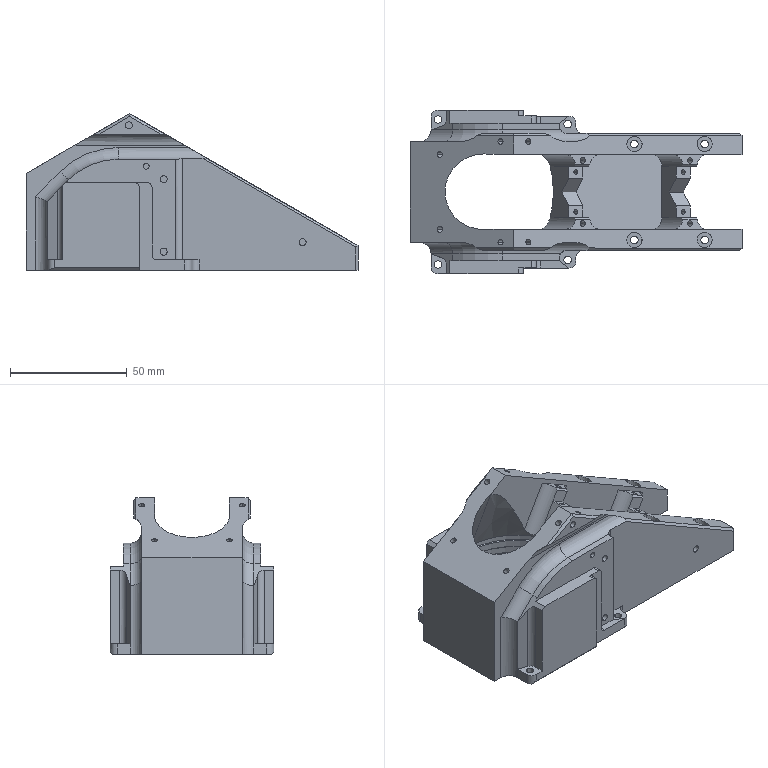NC program | NX | posted with a generic post | part box 142 x 70 x 67 mm
Lines 900 to 2968 of 58889, first 1773 of 2061 lines:
(PLANAR_MILL_COPY_COPY_COPY_COPY_1 , TOOL : D10R0)
N1774 T03 M6
N1776 G54
N1778 G17 G0 G90 X-63.65 Y-40.196 S3500 M3
N1780 G43 Z30.4 H3
N1782 G94 G1 Z-0.6 F5000.
N1784 G3 X-60.65 Y-35. R6. F1800.
N1786 G1 Y-32.472
N1788 X-63.116 Y-31.575
N1790 G3 X-69.024 Y-32.616 R6.
N1792 G0 Z1.4
N1794 X-63.65 Y-40.196
N1796 G1 Z-1.6 F5000.
N1798 G3 X-60.65 Y-35. R6. F1800.
N1800 G1 Y-32.472
N1802 X-63.116 Y-31.575
N1804 G3 X-69.024 Y-32.616 R6.
N1806 G0 Z0.4
N1808 X-63.65 Y-40.196
N1810 G1 Z-2.6 F5000.
N1812 G3 X-60.65 Y-35. R6. F1800.
N1814 G1 Y-32.472
N1816 X-63.116 Y-31.575
N1818 G3 X-69.024 Y-32.616 R6.
N1820 G0 Z-0.6
N1822 X-63.65 Y-40.196
N1824 G1 Z-3.6 F5000.
N1826 G3 X-60.65 Y-35. R6. F1800.
N1828 G1 Y-32.472
N1830 X-63.116 Y-31.574
N1832 G3 X-69.024 Y-32.616 R6.
N1834 G0 Z-1.6
N1836 X-63.65 Y-40.196
N1838 G1 Z-4.6 F5000.
N1840 G3 X-60.65 Y-35. R6. F1800.
N1842 G1 Y-32.472
N1844 X-63.116 Y-31.574
N1846 G3 X-69.024 Y-32.616 R6.
N1848 G0 Z-2.6
N1850 X-63.65 Y-40.196
N1852 G1 Z-5.6 F5000.
N1854 G3 X-60.65 Y-35. R6. F1800.
N1856 G1 Y-32.472
N1858 X-63.116 Y-31.575
N1860 G3 X-69.024 Y-32.616 R6.
N1862 G0 Z-3.6
N1864 X-63.65 Y-40.196
N1866 G1 Z-6.6 F5000.
N1868 G3 X-60.65 Y-35. R6. F1800.
N1870 G1 Y-32.472
N1872 X-63.116 Y-31.574
N1874 G3 X-69.024 Y-32.616 R6.
N1876 G0 Z-4.6
N1878 X-63.65 Y-40.196
N1880 G1 Z-7.6 F5000.
N1882 G3 X-60.65 Y-35. R6. F1800.
N1884 G1 Y-32.472
N1886 X-63.116 Y-31.575
N1888 G3 X-69.024 Y-32.616 R6.
N1890 G0 Z-5.6
N1892 X-63.65 Y-40.196
N1894 G1 Z-8.6 F5000.
N1896 G3 X-60.65 Y-35. R6. F1800.
N1898 G1 Y-32.472
N1900 X-63.116 Y-31.575
N1902 G3 X-69.024 Y-32.616 R6.
N1904 G0 Z-6.6
N1906 X-63.65 Y-40.196
N1908 G1 Z-9.6 F5000.
N1910 G3 X-60.65 Y-35. R6. F1800.
N1912 G1 Y-32.472
N1914 X-63.116 Y-31.575
N1916 G3 X-69.024 Y-32.616 R6.
N1918 G0 Z-7.6
N1920 X-63.65 Y-40.196
N1922 G1 Z-10.6 F5000.
N1924 G3 X-60.65 Y-35. R6. F1800.
N1926 G1 Y-32.472
N1928 X-63.116 Y-31.574
N1930 G3 X-69.024 Y-32.616 R6.
N1932 G0 Z-8.6
N1934 X-63.65 Y-40.196
N1936 G1 Z-11.6 F5000.
N1938 G3 X-60.65 Y-35. R6. F1800.
N1940 G1 Y-32.472
N1942 X-63.116 Y-31.574
N1944 G3 X-69.024 Y-32.616 R6.
N1946 G0 Z-9.6
N1948 X-63.65 Y-40.196
N1950 G1 Z-12.6 F5000.
N1952 G3 X-60.65 Y-35. R6. F1800.
N1954 G1 Y-32.472
N1956 X-63.116 Y-31.575
N1958 G3 X-69.024 Y-32.616 R6.
N1960 G0 Z-10.6
N1962 X-63.65 Y-40.196
N1964 G1 Z-13.6 F5000.
N1966 G3 X-60.65 Y-35. R6. F1800.
N1968 G1 Y-32.472
N1970 X-63.116 Y-31.574
N1972 G3 X-69.024 Y-32.616 R6.
N1974 G0 Z-11.6
N1976 X-63.65 Y-40.196
N1978 G1 Z-14.6 F5000.
N1980 G3 X-60.65 Y-35. R6. F1800.
N1982 G1 Y-32.472
N1984 X-63.116 Y-31.575
N1986 G3 X-69.024 Y-32.616 R6.
N1988 G0 Z-12.6
N1990 X-63.65 Y-40.196
N1992 G1 Z-15.6 F5000.
N1994 G3 X-60.65 Y-35. R6. F1800.
N1996 G1 Y-32.472
N1998 X-63.116 Y-31.575
N2000 G3 X-69.024 Y-32.616 R6.
N2002 G0 Z-13.6
N2004 X-63.65 Y-40.196
N2006 G1 Z-16.6 F5000.
N2008 G3 X-60.65 Y-35. R6. F1800.
N2010 G1 Y-32.472
N2012 X-63.116 Y-31.575
N2014 G3 X-69.024 Y-32.616 R6.
N2016 G0 Z-14.6
N2018 X-63.65 Y-40.196
N2020 G1 Z-17.6 F5000.
N2022 G3 X-60.65 Y-35. R6. F1800.
N2024 G1 Y-32.472
N2026 X-63.116 Y-31.574
N2028 G3 X-69.024 Y-32.616 R6.
N2030 G0 Z-15.6
N2032 X-63.65 Y-40.196
N2034 G1 Z-18.6 F5000.
N2036 G3 X-60.65 Y-35. R6. F1800.
N2038 G1 Y-32.472
N2040 X-63.116 Y-31.574
N2042 G3 X-69.024 Y-32.616 R6.
N2044 G0 Z-16.6
N2046 X-63.65 Y-40.196
N2048 G1 Z-19.6 F5000.
N2050 G3 X-60.65 Y-35. R6. F1800.
N2052 G1 Y-32.472
N2054 X-63.116 Y-31.575
N2056 G3 X-69.024 Y-32.616 R6.
N2058 G0 Z-17.6
N2060 X-63.65 Y-40.196
N2062 G1 Z-20.6 F5000.
N2064 G3 X-60.65 Y-35. R6. F1800.
N2066 G1 Y-32.472
N2068 X-63.116 Y-31.574
N2070 G3 X-69.024 Y-32.616 R6.
N2072 G0 Z-18.6
N2074 X-63.65 Y-40.196
N2076 G1 Z-21.6 F5000.
N2078 G3 X-60.65 Y-35. R6. F1800.
N2080 G1 Y-32.472
N2082 X-63.116 Y-31.575
N2084 G3 X-69.024 Y-32.616 R6.
N2086 G0 Z-19.6
N2088 X-63.65 Y-40.196
N2090 G1 Z-22.6 F5000.
N2092 G3 X-60.65 Y-35. R6. F1800.
N2094 G1 Y-32.472
N2096 X-63.116 Y-31.575
N2098 G3 X-69.024 Y-32.616 R6.
N2100 G0 Z-20.6
N2102 X-63.65 Y-40.196
N2104 G1 Z-23.6 F5000.
N2106 G3 X-60.65 Y-35. R6. F1800.
N2108 G1 Y-32.472
N2110 X-63.116 Y-31.575
N2112 G3 X-69.024 Y-32.616 R6.
N2114 G0 Z-21.6
N2116 X-63.65 Y-40.196
N2118 G1 Z-24.6 F5000.
N2120 G3 X-60.65 Y-35. R6. F1800.
N2122 G1 Y-32.472
N2124 X-63.116 Y-31.574
N2126 G3 X-69.024 Y-32.616 R6.
N2128 G0 Z-22.6
N2130 X-63.65 Y-40.196
N2132 G1 Z-25.6 F5000.
N2134 G3 X-60.65 Y-35. R6. F1800.
N2136 G1 Y-32.472
N2138 X-63.116 Y-31.574
N2140 G3 X-69.024 Y-32.616 R6.
N2142 G0 Z-23.6
N2144 X-63.65 Y-40.196
N2146 G1 Z-26.6 F5000.
N2148 G3 X-60.65 Y-35. R6. F1800.
N2150 G1 Y-32.472
N2152 X-63.116 Y-31.575
N2154 G3 X-69.024 Y-32.616 R6.
N2156 G0 Z-24.6
N2158 X-63.65 Y-40.196
N2160 G1 Z-27.6 F5000.
N2162 G3 X-60.65 Y-35. R6. F1800.
N2164 G1 Y-32.472
N2166 X-63.116 Y-31.574
N2168 G3 X-69.024 Y-32.616 R6.
N2170 G0 Z-25.6
N2172 X-63.65 Y-40.196
N2174 G1 Z-28.6 F5000.
N2176 G3 X-60.65 Y-35. R6. F1800.
N2178 G1 Y-32.472
N2180 X-63.116 Y-31.575
N2182 G3 X-69.024 Y-32.616 R6.
N2184 G0 Z-26.6
N2186 X-63.65 Y-40.196
N2188 G1 Z-29.6 F5000.
N2190 G3 X-60.65 Y-35. R6. F1800.
N2192 G1 Y-32.472
N2194 X-63.116 Y-31.575
N2196 G3 X-69.024 Y-32.616 R6.
N2198 G0 Z-27.6
N2200 X-63.65 Y-40.196
N2202 G1 Z-30.6 F5000.
N2204 G3 X-60.65 Y-35. R6. F1800.
N2206 G1 Y-32.472
N2208 X-63.116 Y-31.575
N2210 G3 X-69.024 Y-32.616 R6.
N2212 G0 Z-28.6
N2214 X-63.65 Y-40.196
N2216 G1 Z-31.6 F5000.
N2218 G3 X-60.65 Y-35. R6. F1800.
N2220 G1 Y-32.472
N2222 X-63.116 Y-31.574
N2224 G3 X-69.024 Y-32.616 R6.
N2226 G0 Z-29.6
N2228 X-63.65 Y-40.196
N2230 G1 Z-32.6 F5000.
N2232 G3 X-60.65 Y-35. R6. F1800.
N2234 G1 Y-32.472
N2236 X-63.116 Y-31.574
N2238 G3 X-69.024 Y-32.616 R6.
N2240 G0 Z-30.6
N2242 X-63.65 Y-40.196
N2244 G1 Z-33.6 F5000.
N2246 G3 X-60.65 Y-35. R6. F1800.
N2248 G1 Y-32.472
N2250 X-63.116 Y-31.575
N2252 G3 X-69.024 Y-32.616 R6.
N2254 G0 Z-31.6
N2256 X-63.65 Y-40.196
N2258 G1 Z-34.6 F5000.
N2260 G3 X-60.65 Y-35. R6. F1800.
N2262 G1 Y-32.472
N2264 X-63.116 Y-31.574
N2266 G3 X-69.024 Y-32.616 R6.
N2268 G0 Z-32.6
N2270 X-63.65 Y-40.196
N2272 G1 Z-35.6 F5000.
N2274 G3 X-60.65 Y-35. R6. F1800.
N2276 G1 Y-32.472
N2278 X-63.116 Y-31.575
N2280 G3 X-69.024 Y-32.616 R6.
N2282 G0 Z-33.6
N2284 X-63.65 Y-40.196
N2286 G1 Z-36.6 F5000.
N2288 G3 X-60.65 Y-35. R6. F1800.
N2290 G1 Y-32.472
N2292 X-63.116 Y-31.575
N2294 G3 X-69.024 Y-32.616 R6.
N2296 G0 Z-34.6
N2298 X-63.65 Y-40.196
N2300 G1 Z-37.6 F5000.
N2302 G3 X-60.65 Y-35. R6. F1800.
N2304 G1 Y-32.472
N2306 X-63.116 Y-31.575
N2308 G3 X-69.024 Y-32.616 R6.
N2310 G0 Z-35.6
N2312 X-63.65 Y-40.196
N2314 G1 Z-38.6 F5000.
N2316 G3 X-60.65 Y-35. R6. F1800.
N2318 G1 Y-32.472
N2320 X-63.116 Y-31.574
N2322 G3 X-69.024 Y-32.616 R6.
N2324 G0 Z-36.6
N2326 X-63.65 Y-40.196
N2328 G1 Z-39.6 F5000.
N2330 G3 X-60.65 Y-35. R6. F1800.
N2332 G1 Y-32.472
N2334 X-63.116 Y-31.574
N2336 G3 X-69.024 Y-32.616 R6.
N2338 G0 Z-37.6
N2340 X-63.65 Y-40.196
N2342 G1 Z-40.6 F5000.
N2344 G3 X-60.65 Y-35. R6. F1800.
N2346 G1 Y-32.472
N2348 X-63.116 Y-31.575
N2350 G3 X-69.024 Y-32.616 R6.
N2352 G0 Z-38.6
N2354 X-63.65 Y-40.196
N2356 G1 Z-41.6 F5000.
N2358 G3 X-60.65 Y-35. R6. F1800.
N2360 G1 Y-32.472
N2362 X-63.116 Y-31.574
N2364 G3 X-69.024 Y-32.616 R6.
N2366 G0 Z-39.6
N2368 X-63.65 Y-40.196
N2370 G1 Z-42.6 F5000.
N2372 G3 X-60.65 Y-35. R6. F1800.
N2374 G1 Y-32.472
N2376 X-63.116 Y-31.575
N2378 G3 X-69.024 Y-32.616 R6.
N2380 G0 Z-40.6
N2382 X-63.65 Y-40.196
N2384 G1 Z-43.6 F5000.
N2386 G3 X-60.65 Y-35. R6. F1800.
N2388 G1 Y-32.472
N2390 X-63.116 Y-31.575
N2392 G3 X-69.024 Y-32.616 R6.
N2394 G0 Z-41.6
N2396 X-63.65 Y-40.196
N2398 G1 Z-44.6 F5000.
N2400 G3 X-60.65 Y-35. R6. F1800.
N2402 G1 Y-32.472
N2404 X-63.116 Y-31.575
N2406 G3 X-69.024 Y-32.616 R6.
N2408 G0 Z-42.6
N2410 X-63.65 Y-40.196
N2412 G1 Z-45.6 F5000.
N2414 G3 X-60.65 Y-35. R6. F1800.
N2416 G1 Y-32.472
N2418 X-63.116 Y-31.574
N2420 G3 X-69.024 Y-32.616 R6.
N2422 G0 Z-43.6
N2424 X-63.65 Y-40.196
N2426 G1 Z-46.6 F5000.
N2428 G3 X-60.65 Y-35. R6. F1800.
N2430 G1 Y-32.472
N2432 X-63.116 Y-31.574
N2434 G3 X-69.024 Y-32.616 R6.
N2436 G0 Z-44.6
N2438 X-63.65 Y-40.196
N2440 G1 Z-47.6 F5000.
N2442 G3 X-60.65 Y-35. R6. F1800.
N2444 G1 Y-32.472
N2446 X-63.116 Y-31.575
N2448 G3 X-69.024 Y-32.616 R6.
N2450 G0 Z-45.6
N2452 X-63.65 Y-40.196
N2454 G1 Z-48.6 F5000.
N2456 G3 X-60.65 Y-35. R6. F1800.
N2458 G1 Y-32.472
N2460 X-63.116 Y-31.574
N2462 G3 X-69.024 Y-32.616 R6.
N2464 G0 Z-46.6
N2466 X-63.65 Y-40.196
N2468 G1 Z-49.6 F5000.
N2470 G3 X-60.65 Y-35. R6. F1800.
N2472 G1 Y-32.472
N2474 X-63.116 Y-31.575
N2476 G3 X-69.024 Y-32.616 R6.
N2478 G0 Z-47.6
N2480 X-63.65 Y-40.196
N2482 G1 Z-50.6 F5000.
N2484 G3 X-60.65 Y-35. R6. F1800.
N2486 G1 Y-32.472
N2488 X-63.116 Y-31.575
N2490 G3 X-69.024 Y-32.616 R6.
N2492 G0 Z-48.6
N2494 X-63.65 Y-40.196
N2496 G1 Z-51.6 F5000.
N2498 G3 X-60.65 Y-35. R6. F1800.
N2500 G1 Y-32.472
N2502 X-63.116 Y-31.575
N2504 G3 X-69.024 Y-32.616 R6.
N2506 G0 Z-49.6
N2508 X-63.65 Y-40.196
N2510 G1 Z-52.6 F5000.
N2512 G3 X-60.65 Y-35. R6. F1800.
N2514 G1 Y-32.472
N2516 X-63.116 Y-31.574
N2518 G3 X-69.024 Y-32.616 R6.
N2520 G0 Z-50.6
N2522 X-63.65 Y-40.196
N2524 G1 Z-53.6 F5000.
N2526 G3 X-60.65 Y-35. R6. F1800.
N2528 G1 Y-32.472
N2530 X-63.116 Y-31.574
N2532 G3 X-69.024 Y-32.616 R6.
N2534 G0 Z-51.6
N2536 X-63.65 Y-40.196
N2538 G1 Z-54.6 F5000.
N2540 G3 X-60.65 Y-35. R6. F1800.
N2542 G1 Y-32.472
N2544 X-63.116 Y-31.575
N2546 G3 X-69.024 Y-32.616 R6.
N2548 G0 Z-52.6
N2550 X-63.65 Y-40.196
N2552 G1 Z-55.6 F5000.
N2554 G3 X-60.65 Y-35. R6. F1800.
N2556 G1 Y-32.472
N2558 X-63.116 Y-31.574
N2560 G3 X-69.024 Y-32.616 R6.
N2562 G0 Z-53.6
N2564 X-63.65 Y-40.196
N2566 G1 Z-56.6 F5000.
N2568 G3 X-60.65 Y-35. R6. F1800.
N2570 G1 Y-32.472
N2572 X-63.116 Y-31.575
N2574 G3 X-69.024 Y-32.616 R6.
N2576 G0 Z-54.6
N2578 X-63.65 Y-40.196
N2580 G1 Z-57.6 F5000.
N2582 G3 X-60.65 Y-35. R6. F1800.
N2584 G1 Y-32.472
N2586 X-63.116 Y-31.575
N2588 G3 X-69.024 Y-32.616 R6.
N2590 G0 Z-55.6
N2592 X-63.65 Y-40.196
N2594 G1 Z-58.6 F5000.
N2596 G3 X-60.65 Y-35. R6. F1800.
N2598 G1 Y-32.472
N2600 X-63.116 Y-31.575
N2602 G3 X-69.024 Y-32.616 R6.
N2604 G0 Z-56.6
N2606 X-63.65 Y-40.196
N2608 G1 Z-59.6 F5000.
N2610 G3 X-60.65 Y-35. R6. F1800.
N2612 G1 Y-32.472
N2614 X-63.116 Y-31.574
N2616 G3 X-69.024 Y-32.616 R6.
N2618 G0 Z-57.6
N2620 X-63.65 Y-40.196
N2622 G1 Z-60.6 F5000.
N2624 G3 X-60.65 Y-35. R6. F1800.
N2626 G1 Y-32.472
N2628 X-63.116 Y-31.574
N2630 G3 X-69.024 Y-32.616 R6.
N2632 G0 Z-58.6
N2634 X-63.65 Y-40.196
N2636 G1 Z-61.6 F5000.
N2638 G3 X-60.65 Y-35. R6. F1800.
N2640 G1 Y-32.472
N2642 X-63.116 Y-31.575
N2644 G3 X-69.024 Y-32.616 R6.
N2646 G0 Z-59.6
N2648 X-63.65 Y-40.196
N2650 G1 Z-62.35 F5000.
N2652 G3 X-60.65 Y-35. R6. F1800.
N2654 G1 Y-32.472
N2656 X-63.116 Y-31.574
N2658 G3 X-69.024 Y-32.616 R6.
N2660 G0 Z30.4
N2662 Y32.616
N2664 G1 Z-0.6 F5000.
N2666 G3 X-63.116 Y31.575 R6. F1800.
N2668 G1 X-60.65 Y32.472
N2670 Y35.
N2672 G3 X-63.65 Y40.196 R6.
N2674 G0 Z1.4
N2676 X-69.024 Y32.616
N2678 G1 Z-1.6 F5000.
N2680 G3 X-63.116 Y31.575 R6. F1800.
N2682 G1 X-60.65 Y32.472
N2684 Y35.
N2686 G3 X-63.65 Y40.196 R6.
N2688 G0 Z0.4
N2690 X-69.024 Y32.616
N2692 G1 Z-2.6 F5000.
N2694 G3 X-63.116 Y31.574 R6. F1800.
N2696 G1 X-60.65 Y32.472
N2698 Y35.
N2700 G3 X-63.65 Y40.196 R6.
N2702 G0 Z-0.6
N2704 X-69.024 Y32.616
N2706 G1 Z-3.6 F5000.
N2708 G3 X-63.116 Y31.575 R6. F1800.
N2710 G1 X-60.65 Y32.472
N2712 Y35.
N2714 G3 X-63.65 Y40.196 R6.
N2716 G0 Z-1.6
N2718 X-69.024 Y32.616
N2720 G1 Z-4.6 F5000.
N2722 G3 X-63.116 Y31.575 R6. F1800.
N2724 G1 X-60.65 Y32.472
N2726 Y35.
N2728 G3 X-63.65 Y40.196 R6.
N2730 G0 Z-2.6
N2732 X-69.024 Y32.616
N2734 G1 Z-5.6 F5000.
N2736 G3 X-63.116 Y31.575 R6. F1800.
N2738 G1 X-60.65 Y32.472
N2740 Y35.
N2742 G3 X-63.65 Y40.196 R6.
N2744 G0 Z-3.6
N2746 X-69.024 Y32.616
N2748 G1 Z-6.6 F5000.
N2750 G3 X-63.116 Y31.575 R6. F1800.
N2752 G1 X-60.65 Y32.472
N2754 Y35.
N2756 G3 X-63.65 Y40.196 R6.
N2758 G0 Z-4.6
N2760 X-69.024 Y32.616
N2762 G1 Z-7.6 F5000.
N2764 G3 X-63.116 Y31.575 R6. F1800.
N2766 G1 X-60.65 Y32.472
N2768 Y35.
N2770 G3 X-63.65 Y40.196 R6.
N2772 G0 Z-5.6
N2774 X-69.024 Y32.616
N2776 G1 Z-8.6 F5000.
N2778 G3 X-63.116 Y31.575 R6. F1800.
N2780 G1 X-60.65 Y32.472
N2782 Y35.
N2784 G3 X-63.65 Y40.196 R6.
N2786 G0 Z-6.6
N2788 X-69.024 Y32.616
N2790 G1 Z-9.6 F5000.
N2792 G3 X-63.116 Y31.574 R6. F1800.
N2794 G1 X-60.65 Y32.472
N2796 Y35.
N2798 G3 X-63.65 Y40.196 R6.
N2800 G0 Z-7.6
N2802 X-69.024 Y32.616
N2804 G1 Z-10.6 F5000.
N2806 G3 X-63.116 Y31.575 R6. F1800.
N2808 G1 X-60.65 Y32.472
N2810 Y35.
N2812 G3 X-63.65 Y40.196 R6.
N2814 G0 Z-8.6
N2816 X-69.024 Y32.616
N2818 G1 Z-11.6 F5000.
N2820 G3 X-63.116 Y31.575 R6. F1800.
N2822 G1 X-60.65 Y32.472
N2824 Y35.
N2826 G3 X-63.65 Y40.196 R6.
N2828 G0 Z-9.6
N2830 X-69.024 Y32.616
N2832 G1 Z-12.6 F5000.
N2834 G3 X-63.116 Y31.575 R6. F1800.
N2836 G1 X-60.65 Y32.472
N2838 Y35.
N2840 G3 X-63.65 Y40.196 R6.
N2842 G0 Z-10.6
N2844 X-69.024 Y32.616
N2846 G1 Z-13.6 F5000.
N2848 G3 X-63.116 Y31.575 R6. F1800.
N2850 G1 X-60.65 Y32.472
N2852 Y35.
N2854 G3 X-63.65 Y40.196 R6.
N2856 G0 Z-11.6
N2858 X-69.024 Y32.616
N2860 G1 Z-14.6 F5000.
N2862 G3 X-63.116 Y31.575 R6. F1800.
N2864 G1 X-60.65 Y32.472
N2866 Y35.
N2868 G3 X-63.65 Y40.196 R6.
N2870 G0 Z-12.6
N2872 X-69.024 Y32.616
N2874 G1 Z-15.6 F5000.
N2876 G3 X-63.116 Y31.575 R6. F1800.
N2878 G1 X-60.65 Y32.472
N2880 Y35.
N2882 G3 X-63.65 Y40.196 R6.
N2884 G0 Z-13.6
N2886 X-69.024 Y32.616
N2888 G1 Z-16.6 F5000.
N2890 G3 X-63.116 Y31.574 R6. F1800.
N2892 G1 X-60.65 Y32.472
N2894 Y35.
N2896 G3 X-63.65 Y40.196 R6.
N2898 G0 Z-14.6
N2900 X-69.024 Y32.616
N2902 G1 Z-17.6 F5000.
N2904 G3 X-63.116 Y31.575 R6. F1800.
N2906 G1 X-60.65 Y32.472
N2908 Y35.
N2910 G3 X-63.65 Y40.196 R6.
N2912 G0 Z-15.6
N2914 X-69.024 Y32.616
N2916 G1 Z-18.6 F5000.
N2918 G3 X-63.116 Y31.575 R6. F1800.
N2920 G1 X-60.65 Y32.472
N2922 Y35.
N2924 G3 X-63.65 Y40.196 R6.
N2926 G0 Z-16.6
N2928 X-69.024 Y32.616
N2930 G1 Z-19.6 F5000.
N2932 G3 X-63.116 Y31.575 R6. F1800.
N2934 G1 X-60.65 Y32.472
N2936 Y35.
N2938 G3 X-63.65 Y40.196 R6.
N2940 G0 Z-17.6
N2942 X-69.024 Y32.616
N2944 G1 Z-20.6 F5000.
N2946 G3 X-63.116 Y31.575 R6. F1800.
N2948 G1 X-60.65 Y32.472
N2950 Y35.
N2952 G3 X-63.65 Y40.196 R6.
N2954 G0 Z-18.6
N2956 X-69.024 Y32.616
N2958 G1 Z-21.6 F5000.
N2960 G3 X-63.116 Y31.575 R6. F1800.
N2962 G1 X-60.65 Y32.472
N2964 Y35.
N2966 G3 X-63.65 Y40.196 R6.
N2968 G0 Z-19.6
N2970 X-69.024 Y32.616
N2972 G1 Z-22.6 F5000.
N2974 G3 X-63.116 Y31.575 R6. F1800.
N2976 G1 X-60.65 Y32.472
N2978 Y35.
N2980 G3 X-63.65 Y40.196 R6.
N2982 G0 Z-20.6
N2984 X-69.024 Y32.616
N2986 G1 Z-23.6 F5000.
N2988 G3 X-63.116 Y31.574 R6. F1800.
N2990 G1 X-60.65 Y32.472
N2992 Y35.
N2994 G3 X-63.65 Y40.196 R6.
N2996 G0 Z-21.6
N2998 X-69.024 Y32.616
N3000 G1 Z-24.6 F5000.
N3002 G3 X-63.116 Y31.575 R6. F1800.
N3004 G1 X-60.65 Y32.472
N3006 Y35.
N3008 G3 X-63.65 Y40.196 R6.
N3010 G0 Z-22.6
N3012 X-69.024 Y32.616
N3014 G1 Z-25.6 F5000.
N3016 G3 X-63.116 Y31.575 R6. F1800.
N3018 G1 X-60.65 Y32.472
N3020 Y35.
N3022 G3 X-63.65 Y40.196 R6.
N3024 G0 Z-23.6
N3026 X-69.024 Y32.616
N3028 G1 Z-26.6 F5000.
N3030 G3 X-63.116 Y31.575 R6. F1800.
N3032 G1 X-60.65 Y32.472
N3034 Y35.
N3036 G3 X-63.65 Y40.196 R6.
N3038 G0 Z-24.6
N3040 X-69.024 Y32.616
N3042 G1 Z-27.6 F5000.
N3044 G3 X-63.116 Y31.575 R6. F1800.
N3046 G1 X-60.65 Y32.472
N3048 Y35.
N3050 G3 X-63.65 Y40.196 R6.
N3052 G0 Z-25.6
N3054 X-69.024 Y32.616
N3056 G1 Z-28.6 F5000.
N3058 G3 X-63.116 Y31.575 R6. F1800.
N3060 G1 X-60.65 Y32.472
N3062 Y35.
N3064 G3 X-63.65 Y40.196 R6.
N3066 G0 Z-26.6
N3068 X-69.024 Y32.616
N3070 G1 Z-29.6 F5000.
N3072 G3 X-63.116 Y31.575 R6. F1800.
N3074 G1 X-60.65 Y32.472
N3076 Y35.
N3078 G3 X-63.65 Y40.196 R6.
N3080 G0 Z-27.6
N3082 X-69.024 Y32.616
N3084 G1 Z-30.6 F5000.
N3086 G3 X-63.116 Y31.574 R6. F1800.
N3088 G1 X-60.65 Y32.472
N3090 Y35.
N3092 G3 X-63.65 Y40.196 R6.
N3094 G0 Z-28.6
N3096 X-69.024 Y32.616
N3098 G1 Z-31.6 F5000.
N3100 G3 X-63.116 Y31.575 R6. F1800.
N3102 G1 X-60.65 Y32.472
N3104 Y35.
N3106 G3 X-63.65 Y40.196 R6.
N3108 G0 Z-29.6
N3110 X-69.024 Y32.616
N3112 G1 Z-32.6 F5000.
N3114 G3 X-63.116 Y31.575 R6. F1800.
N3116 G1 X-60.65 Y32.472
N3118 Y35.
N3120 G3 X-63.65 Y40.196 R6.
N3122 G0 Z-30.6
N3124 X-69.024 Y32.616
N3126 G1 Z-33.6 F5000.
N3128 G3 X-63.116 Y31.575 R6. F1800.
N3130 G1 X-60.65 Y32.472
N3132 Y35.
N3134 G3 X-63.65 Y40.196 R6.
N3136 G0 Z-31.6
N3138 X-69.024 Y32.616
N3140 G1 Z-34.6 F5000.
N3142 G3 X-63.116 Y31.575 R6. F1800.
N3144 G1 X-60.65 Y32.472
N3146 Y35.
N3148 G3 X-63.65 Y40.196 R6.
N3150 G0 Z-32.6
N3152 X-69.024 Y32.616
N3154 G1 Z-35.6 F5000.
N3156 G3 X-63.116 Y31.575 R6. F1800.
N3158 G1 X-60.65 Y32.472
N3160 Y35.
N3162 G3 X-63.65 Y40.196 R6.
N3164 G0 Z-33.6
N3166 X-69.024 Y32.616
N3168 G1 Z-36.6 F5000.
N3170 G3 X-63.116 Y31.575 R6. F1800.
N3172 G1 X-60.65 Y32.472
N3174 Y35.
N3176 G3 X-63.65 Y40.196 R6.
N3178 G0 Z-34.6
N3180 X-69.024 Y32.616
N3182 G1 Z-37.6 F5000.
N3184 G3 X-63.116 Y31.574 R6. F1800.
N3186 G1 X-60.65 Y32.472
N3188 Y35.
N3190 G3 X-63.65 Y40.196 R6.
N3192 G0 Z-35.6
N3194 X-69.024 Y32.616
N3196 G1 Z-38.6 F5000.
N3198 G3 X-63.116 Y31.575 R6. F1800.
N3200 G1 X-60.65 Y32.472
N3202 Y35.
N3204 G3 X-63.65 Y40.196 R6.
N3206 G0 Z-36.6
N3208 X-69.024 Y32.616
N3210 G1 Z-39.6 F5000.
N3212 G3 X-63.116 Y31.575 R6. F1800.
N3214 G1 X-60.65 Y32.472
N3216 Y35.
N3218 G3 X-63.65 Y40.196 R6.
N3220 G0 Z-37.6
N3222 X-69.024 Y32.616
N3224 G1 Z-40.6 F5000.
N3226 G3 X-63.116 Y31.575 R6. F1800.
N3228 G1 X-60.65 Y32.472
N3230 Y35.
N3232 G3 X-63.65 Y40.196 R6.
N3234 G0 Z-38.6
N3236 X-69.024 Y32.616
N3238 G1 Z-41.6 F5000.
N3240 G3 X-63.116 Y31.575 R6. F1800.
N3242 G1 X-60.65 Y32.472
N3244 Y35.
N3246 G3 X-63.65 Y40.196 R6.
N3248 G0 Z-39.6
N3250 X-69.024 Y32.616
N3252 G1 Z-42.6 F5000.
N3254 G3 X-63.116 Y31.575 R6. F1800.
N3256 G1 X-60.65 Y32.472
N3258 Y35.
N3260 G3 X-63.65 Y40.196 R6.
N3262 G0 Z-40.6
N3264 X-69.024 Y32.616
N3266 G1 Z-43.6 F5000.
N3268 G3 X-63.116 Y31.575 R6. F1800.
N3270 G1 X-60.65 Y32.472
N3272 Y35.
N3274 G3 X-63.65 Y40.196 R6.
N3276 G0 Z-41.6
N3278 X-69.024 Y32.616
N3280 G1 Z-44.6 F5000.
N3282 G3 X-63.116 Y31.574 R6. F1800.
N3284 G1 X-60.65 Y32.472
N3286 Y35.
N3288 G3 X-63.65 Y40.196 R6.
N3290 G0 Z-42.6
N3292 X-69.024 Y32.616
N3294 G1 Z-45.6 F5000.
N3296 G3 X-63.116 Y31.575 R6. F1800.
N3298 G1 X-60.65 Y32.472
N3300 Y35.
N3302 G3 X-63.65 Y40.196 R6.
N3304 G0 Z-43.6
N3306 X-69.024 Y32.616
N3308 G1 Z-46.6 F5000.
N3310 G3 X-63.116 Y31.575 R6. F1800.
N3312 G1 X-60.65 Y32.472
N3314 Y35.
N3316 G3 X-63.65 Y40.196 R6.
N3318 G0 Z-44.6
N3320 X-69.024 Y32.616
N3322 G1 Z-47.6 F5000.
N3324 G3 X-63.116 Y31.575 R6. F1800.
N3326 G1 X-60.65 Y32.472
N3328 Y35.
N3330 G3 X-63.65 Y40.196 R6.
N3332 G0 Z-45.6
N3334 X-69.024 Y32.616
N3336 G1 Z-48.6 F5000.
N3338 G3 X-63.116 Y31.575 R6. F1800.
N3340 G1 X-60.65 Y32.472
N3342 Y35.
N3344 G3 X-63.65 Y40.196 R6.
N3346 G0 Z-46.6
N3348 X-69.024 Y32.616
N3350 G1 Z-49.6 F5000.
N3352 G3 X-63.116 Y31.575 R6. F1800.
N3354 G1 X-60.65 Y32.472
N3356 Y35.
N3358 G3 X-63.65 Y40.196 R6.
N3360 G0 Z-47.6
N3362 X-69.024 Y32.616
N3364 G1 Z-50.6 F5000.
N3366 G3 X-63.116 Y31.575 R6. F1800.
N3368 G1 X-60.65 Y32.472
N3370 Y35.
N3372 G3 X-63.65 Y40.196 R6.
N3374 G0 Z-48.6
N3376 X-69.024 Y32.616
N3378 G1 Z-51.6 F5000.
N3380 G3 X-63.116 Y31.574 R6. F1800.
N3382 G1 X-60.65 Y32.472
N3384 Y35.
N3386 G3 X-63.65 Y40.196 R6.
N3388 G0 Z-49.6
N3390 X-69.024 Y32.616
N3392 G1 Z-52.6 F5000.
N3394 G3 X-63.116 Y31.575 R6. F1800.
N3396 G1 X-60.65 Y32.472
N3398 Y35.
N3400 G3 X-63.65 Y40.196 R6.
N3402 G0 Z-50.6
N3404 X-69.024 Y32.616
N3406 G1 Z-53.6 F5000.
N3408 G3 X-63.116 Y31.575 R6. F1800.
N3410 G1 X-60.65 Y32.472
N3412 Y35.
N3414 G3 X-63.65 Y40.196 R6.
N3416 G0 Z-51.6
N3418 X-69.024 Y32.616
N3420 G1 Z-54.6 F5000.
N3422 G3 X-63.116 Y31.575 R6. F1800.
N3424 G1 X-60.65 Y32.472
N3426 Y35.
N3428 G3 X-63.65 Y40.196 R6.
N3430 G0 Z-52.6
N3432 X-69.024 Y32.616
N3434 G1 Z-55.6 F5000.
N3436 G3 X-63.116 Y31.575 R6. F1800.
N3438 G1 X-60.65 Y32.472
N3440 Y35.
N3442 G3 X-63.65 Y40.196 R6.
N3444 G0 Z-53.6
N3446 X-69.024 Y32.616
N3448 G1 Z-56.6 F5000.
N3450 G3 X-63.116 Y31.575 R6. F1800.
N3452 G1 X-60.65 Y32.472
N3454 Y35.
N3456 G3 X-63.65 Y40.196 R6.
N3458 G0 Z-54.6
N3460 X-69.024 Y32.616
N3462 G1 Z-57.6 F5000.
N3464 G3 X-63.116 Y31.575 R6. F1800.
N3466 G1 X-60.65 Y32.472
N3468 Y35.
N3470 G3 X-63.65 Y40.196 R6.
N3472 G0 Z-55.6
N3474 X-69.024 Y32.616
N3476 G1 Z-58.6 F5000.
N3478 G3 X-63.116 Y31.574 R6. F1800.
N3480 G1 X-60.65 Y32.472
N3482 Y35.
N3484 G3 X-63.65 Y40.196 R6.
N3486 G0 Z-56.6
N3488 X-69.024 Y32.616
N3490 G1 Z-59.6 F5000.
N3492 G3 X-63.116 Y31.575 R6. F1800.
N3494 G1 X-60.65 Y32.472
N3496 Y35.
N3498 G3 X-63.65 Y40.196 R6.
N3500 G0 Z-57.6
N3502 X-69.024 Y32.616
N3504 G1 Z-60.6 F5000.
N3506 G3 X-63.116 Y31.575 R6. F1800.
N3508 G1 X-60.65 Y32.472
N3510 Y35.
N3512 G3 X-63.65 Y40.196 R6.
N3514 G0 Z-58.6
N3516 X-69.024 Y32.616
N3518 G1 Z-61.6 F5000.
N3520 G3 X-63.116 Y31.575 R6. F1800.
N3522 G1 X-60.65 Y32.472
N3524 Y35.
N3526 G3 X-63.65 Y40.196 R6.
N3528 G0 Z-59.6
N3530 X-69.024 Y32.616
N3532 G1 Z-62.35 F5000.
N3534 G3 X-63.116 Y31.575 R6. F1800.
N3536 G1 X-60.65 Y32.472
N3538 Y35.
N3540 G3 X-63.65 Y40.196 R6.
N3542 G0 Z30.4
(PLANAR_MILL_COPY_COPY_COPY_COPY_1_COPY , TOOL : D10R0)
N3544 X1.05 Y38.096
N3546 Z30.
N3548 G1 Z-1. F5000.
N3550 G3 X-1.95 Y32.9 R6. F1800.
N3552 G1 Y30.15
N3554 X8.
N3556 G3 X13.196 Y33.15 R6.
N3558 G0 Z1.
N3560 X1.05 Y38.096
N3562 G1 Z-2. F5000.
N3564 G3 X-1.95 Y32.9 R6. F1800.
N3566 G1 Y30.15
N3568 X8.
N3570 G3 X13.196 Y33.15 R6.
N3572 G0 Z0.
N3574 X1.05 Y38.096
N3576 G1 Z-3. F5000.
N3578 G3 X-1.95 Y32.9 R6. F1800.
N3580 G1 Y30.15
N3582 X8.
N3584 G3 X13.196 Y33.15 R6.
N3586 G0 Z-1.
N3588 X1.05 Y38.096
N3590 G1 Z-4. F5000.
N3592 G3 X-1.95 Y32.9 R6. F1800.
N3594 G1 Y30.15
N3596 X8.
N3598 G3 X13.196 Y33.15 R6.
N3600 G0 Z-2.
N3602 X1.05 Y38.096
N3604 G1 Z-5. F5000.
N3606 G3 X-1.95 Y32.9 R6. F1800.
N3608 G1 Y30.15
N3610 X8.
N3612 G3 X13.196 Y33.15 R6.
N3614 G0 Z-3.
N3616 X1.05 Y38.096
N3618 G1 Z-6. F5000.
N3620 G3 X-1.95 Y32.9 R6. F1800.
N3622 G1 Y30.15
N3624 X8.
N3626 G3 X13.196 Y33.15 R6.
N3628 G0 Z-4.
N3630 X1.05 Y38.096
N3632 G1 Z-7. F5000.
N3634 G3 X-1.95 Y32.9 R6. F1800.
N3636 G1 Y30.15
N3638 X8.
N3640 G3 X13.196 Y33.15 R6.
N3642 G0 Z-5.
N3644 X1.05 Y38.096
N3646 G1 Z-8. F5000.
N3648 G3 X-1.95 Y32.9 R6. F1800.
N3650 G1 Y30.15
N3652 X8.
N3654 G3 X13.196 Y33.15 R6.
N3656 G0 Z-6.
N3658 X1.05 Y38.096
N3660 G1 Z-9. F5000.
N3662 G3 X-1.95 Y32.9 R6. F1800.
N3664 G1 Y30.15
N3666 X8.
N3668 G3 X13.196 Y33.15 R6.
N3670 G0 Z-7.
N3672 X1.05 Y38.096
N3674 G1 Z-10. F5000.
N3676 G3 X-1.95 Y32.9 R6. F1800.
N3678 G1 Y30.15
N3680 X8.
N3682 G3 X13.196 Y33.15 R6.
N3684 G0 Z-8.
N3686 X1.05 Y38.096
N3688 G1 Z-11. F5000.
N3690 G3 X-1.95 Y32.9 R6. F1800.
N3692 G1 Y30.15
N3694 X8.
N3696 G3 X13.196 Y33.15 R6.
N3698 G0 Z-9.
N3700 X1.05 Y38.096
N3702 G1 Z-12. F5000.
N3704 G3 X-1.95 Y32.9 R6. F1800.
N3706 G1 Y30.15
N3708 X8.
N3710 G3 X13.196 Y33.15 R6.
N3712 G0 Z-10.
N3714 X1.05 Y38.096
N3716 G1 Z-13. F5000.
N3718 G3 X-1.95 Y32.9 R6. F1800.
N3720 G1 Y30.15
N3722 X8.
N3724 G3 X13.196 Y33.15 R6.
N3726 G0 Z-11.
N3728 X1.05 Y38.096
N3730 G1 Z-14. F5000.
N3732 G3 X-1.95 Y32.9 R6. F1800.
N3734 G1 Y30.15
N3736 X8.
N3738 G3 X13.196 Y33.15 R6.
N3740 G0 Z-12.
N3742 X1.05 Y38.096
N3744 G1 Z-15. F5000.
N3746 G3 X-1.95 Y32.9 R6. F1800.
N3748 G1 Y30.15
N3750 X8.
N3752 G3 X13.196 Y33.15 R6.
N3754 G0 Z-13.
N3756 X1.05 Y38.096
N3758 G1 Z-16. F5000.
N3760 G3 X-1.95 Y32.9 R6. F1800.
N3762 G1 Y30.15
N3764 X8.
N3766 G3 X13.196 Y33.15 R6.
N3768 G0 Z-14.
N3770 X1.05 Y38.096
N3772 G1 Z-17. F5000.
N3774 G3 X-1.95 Y32.9 R6. F1800.
N3776 G1 Y30.15
N3778 X8.
N3780 G3 X13.196 Y33.15 R6.
N3782 G0 Z-15.
N3784 X1.05 Y38.096
N3786 G1 Z-18. F5000.
N3788 G3 X-1.95 Y32.9 R6. F1800.
N3790 G1 Y30.15
N3792 X8.
N3794 G3 X13.196 Y33.15 R6.
N3796 G0 Z-16.
N3798 X1.05 Y38.096
N3800 G1 Z-19. F5000.
N3802 G3 X-1.95 Y32.9 R6. F1800.
N3804 G1 Y30.15
N3806 X8.
N3808 G3 X13.196 Y33.15 R6.
N3810 G0 Z-17.
N3812 X1.05 Y38.096
N3814 G1 Z-20. F5000.
N3816 G3 X-1.95 Y32.9 R6. F1800.
N3818 G1 Y30.15
N3820 X8.
N3822 G3 X13.196 Y33.15 R6.
N3824 G0 Z-18.
N3826 X1.05 Y38.096
N3828 G1 Z-21. F5000.
N3830 G3 X-1.95 Y32.9 R6. F1800.
N3832 G1 Y30.15
N3834 X8.
N3836 G3 X13.196 Y33.15 R6.
N3838 G0 Z-19.
N3840 X1.05 Y38.096
N3842 G1 Z-22. F5000.
N3844 G3 X-1.95 Y32.9 R6. F1800.
N3846 G1 Y30.15
N3848 X8.
N3850 G3 X13.196 Y33.15 R6.
N3852 G0 Z-20.
N3854 X1.05 Y38.096
N3856 G1 Z-23. F5000.
N3858 G3 X-1.95 Y32.9 R6. F1800.
N3860 G1 Y30.15
N3862 X8.
N3864 G3 X13.196 Y33.15 R6.
N3866 G0 Z-21.
N3868 X1.05 Y38.096
N3870 G1 Z-24. F5000.
N3872 G3 X-1.95 Y32.9 R6. F1800.
N3874 G1 Y30.15
N3876 X8.
N3878 G3 X13.196 Y33.15 R6.
N3880 G0 Z-22.
N3882 X1.05 Y38.096
N3884 G1 Z-25. F5000.
N3886 G3 X-1.95 Y32.9 R6. F1800.
N3888 G1 Y30.15
N3890 X8.
N3892 G3 X13.196 Y33.15 R6.
N3894 G0 Z-23.
N3896 X1.05 Y38.096
N3898 G1 Z-26. F5000.
N3900 G3 X-1.95 Y32.9 R6. F1800.
N3902 G1 Y30.15
N3904 X8.
N3906 G3 X13.196 Y33.15 R6.
N3908 G0 Z-24.
N3910 X1.05 Y38.096
N3912 G1 Z-27. F5000.
N3914 G3 X-1.95 Y32.9 R6. F1800.
N3916 G1 Y30.15
N3918 X8.
N3920 G3 X13.196 Y33.15 R6.
N3922 G0 Z-25.
N3924 X1.05 Y38.096
N3926 G1 Z-28. F5000.
N3928 G3 X-1.95 Y32.9 R6. F1800.
N3930 G1 Y30.15
N3932 X8.
N3934 G3 X13.196 Y33.15 R6.
N3936 G0 Z-26.
N3938 X1.05 Y38.096
N3940 G1 Z-29. F5000.
N3942 G3 X-1.95 Y32.9 R6. F1800.
N3944 G1 Y30.15
N3946 X8.
N3948 G3 X13.196 Y33.15 R6.
N3950 G0 Z-27.
N3952 X1.05 Y38.096
N3954 G1 Z-30. F5000.
N3956 G3 X-1.95 Y32.9 R6. F1800.
N3958 G1 Y30.15
N3960 X8.
N3962 G3 X13.196 Y33.15 R6.
N3964 G0 Z-28.
N3966 X1.05 Y38.096
N3968 G1 Z-31. F5000.
N3970 G3 X-1.95 Y32.9 R6. F1800.
N3972 G1 Y30.15
N3974 X8.
N3976 G3 X13.196 Y33.15 R6.
N3978 G0 Z-29.
N3980 X1.05 Y38.096
N3982 G1 Z-32. F5000.
N3984 G3 X-1.95 Y32.9 R6. F1800.
N3986 G1 Y30.15
N3988 X8.
N3990 G3 X13.196 Y33.15 R6.
N3992 G0 Z-30.
N3994 X1.05 Y38.096
N3996 G1 Z-33. F5000.
N3998 G3 X-1.95 Y32.9 R6. F1800.
N4000 G1 Y30.15
N4002 X8.
N4004 G3 X13.196 Y33.15 R6.
N4006 G0 Z-31.
N4008 X1.05 Y38.096
N4010 G1 Z-34. F5000.
N4012 G3 X-1.95 Y32.9 R6. F1800.
N4014 G1 Y30.15
N4016 X8.
N4018 G3 X13.196 Y33.15 R6.
N4020 G0 Z-32.
N4022 X1.05 Y38.096
N4024 G1 Z-35. F5000.
N4026 G3 X-1.95 Y32.9 R6. F1800.
N4028 G1 Y30.15
N4030 X8.
N4032 G3 X13.196 Y33.15 R6.
N4034 G0 Z-33.
N4036 X1.05 Y38.096
N4038 G1 Z-36. F5000.
N4040 G3 X-1.95 Y32.9 R6. F1800.
N4042 G1 Y30.15
N4044 X8.
N4046 G3 X13.196 Y33.15 R6.
N4048 G0 Z-34.
N4050 X1.05 Y38.096
N4052 G1 Z-37. F5000.
N4054 G3 X-1.95 Y32.9 R6. F1800.
N4056 G1 Y30.15
N4058 X8.
N4060 G3 X13.196 Y33.15 R6.
N4062 G0 Z-35.
N4064 X1.05 Y38.096
N4066 G1 Z-38. F5000.
N4068 G3 X-1.95 Y32.9 R6. F1800.
N4070 G1 Y30.15
N4072 X8.
N4074 G3 X13.196 Y33.15 R6.
N4076 G0 Z-36.
N4078 X1.05 Y38.096
N4080 G1 Z-39. F5000.
N4082 G3 X-1.95 Y32.9 R6. F1800.
N4084 G1 Y30.15
N4086 X8.
N4088 G3 X13.196 Y33.15 R6.
N4090 G0 Z-37.
N4092 X1.05 Y38.096
N4094 G1 Z-40. F5000.
N4096 G3 X-1.95 Y32.9 R6. F1800.
N4098 G1 Y30.15
N4100 X8.
N4102 G3 X13.196 Y33.15 R6.
N4104 G0 Z-38.
N4106 X1.05 Y38.096
N4108 G1 Z-41. F5000.
N4110 G3 X-1.95 Y32.9 R6. F1800.
N4112 G1 Y30.15
N4114 X8.
N4116 G3 X13.196 Y33.15 R6.
N4118 G0 Z-39.
N4120 X1.05 Y38.096
N4122 G1 Z-42. F5000.
N4124 G3 X-1.95 Y32.9 R6. F1800.
N4126 G1 Y30.15
N4128 X8.
N4130 G3 X13.196 Y33.15 R6.
N4132 G0 Z-40.
N4134 X1.05 Y38.096
N4136 G1 Z-43. F5000.
N4138 G3 X-1.95 Y32.9 R6. F1800.
N4140 G1 Y30.15
N4142 X8.
N4144 G3 X13.196 Y33.15 R6.
N4146 G0 Z-41.
N4148 X1.05 Y38.096
N4150 G1 Z-44. F5000.
N4152 G3 X-1.95 Y32.9 R6. F1800.
N4154 G1 Y30.15
N4156 X8.
N4158 G3 X13.196 Y33.15 R6.
N4160 G0 Z-42.
N4162 X1.05 Y38.096
N4164 G1 Z-45. F5000.
N4166 G3 X-1.95 Y32.9 R6. F1800.
N4168 G1 Y30.15
N4170 X8.
N4172 G3 X13.196 Y33.15 R6.
N4174 G0 Z-43.
N4176 X1.05 Y38.096
N4178 G1 Z-46. F5000.
N4180 G3 X-1.95 Y32.9 R6. F1800.
N4182 G1 Y30.15
N4184 X8.
N4186 G3 X13.196 Y33.15 R6.
N4188 G0 Z-44.
N4190 X1.05 Y38.096
N4192 G1 Z-47. F5000.
N4194 G3 X-1.95 Y32.9 R6. F1800.
N4196 G1 Y30.15
N4198 X8.
N4200 G3 X13.196 Y33.15 R6.
N4202 G0 Z-45.
N4204 X1.05 Y38.096
N4206 G1 Z-48. F5000.
N4208 G3 X-1.95 Y32.9 R6. F1800.
N4210 G1 Y30.15
N4212 X8.
N4214 G3 X13.196 Y33.15 R6.
N4216 G0 Z-46.
N4218 X1.05 Y38.096
N4220 G1 Z-49. F5000.
N4222 G3 X-1.95 Y32.9 R6. F1800.
N4224 G1 Y30.15
N4226 X8.
N4228 G3 X13.196 Y33.15 R6.
N4230 G0 Z-47.
N4232 X1.05 Y38.096
N4234 G1 Z-50. F5000.
N4236 G3 X-1.95 Y32.9 R6. F1800.
N4238 G1 Y30.15
N4240 X8.
N4242 G3 X13.196 Y33.15 R6.
N4244 G0 Z-48.
N4246 X1.05 Y38.096
N4248 G1 Z-51. F5000.
N4250 G3 X-1.95 Y32.9 R6. F1800.
N4252 G1 Y30.15
N4254 X8.
N4256 G3 X13.196 Y33.15 R6.
N4258 G0 Z-49.
N4260 X1.05 Y38.096
N4262 G1 Z-52. F5000.
N4264 G3 X-1.95 Y32.9 R6. F1800.
N4266 G1 Y30.15
N4268 X8.
N4270 G3 X13.196 Y33.15 R6.
N4272 G0 Z-50.
N4274 X1.05 Y38.096
N4276 G1 Z-53. F5000.
N4278 G3 X-1.95 Y32.9 R6. F1800.
N4280 G1 Y30.15
N4282 X8.
N4284 G3 X13.196 Y33.15 R6.
N4286 G0 Z-51.
N4288 X1.05 Y38.096
N4290 G1 Z-54. F5000.
N4292 G3 X-1.95 Y32.9 R6. F1800.
N4294 G1 Y30.15
N4296 X8.
N4298 G3 X13.196 Y33.15 R6.
N4300 G0 Z-52.
N4302 X1.05 Y38.096
N4304 G1 Z-55. F5000.
N4306 G3 X-1.95 Y32.9 R6. F1800.
N4308 G1 Y30.15
N4310 X8.
N4312 G3 X13.196 Y33.15 R6.
N4314 G0 Z-53.
N4316 X1.05 Y38.096
N4318 G1 Z-56. F5000.
N4320 G3 X-1.95 Y32.9 R6. F1800.
N4322 G1 Y30.15
N4324 X8.
N4326 G3 X13.196 Y33.15 R6.
N4328 G0 Z-54.
N4330 X1.05 Y38.096
N4332 G1 Z-57. F5000.
N4334 G3 X-1.95 Y32.9 R6. F1800.
N4336 G1 Y30.15
N4338 X8.
N4340 G3 X13.196 Y33.15 R6.
N4342 G0 Z-55.
N4344 X1.05 Y38.096
N4346 G1 Z-58. F5000.
N4348 G3 X-1.95 Y32.9 R6. F1800.
N4350 G1 Y30.15
N4352 X8.
N4354 G3 X13.196 Y33.15 R6.
N4356 G0 Z-56.
N4358 X1.05 Y38.096
N4360 G1 Z-59. F5000.
N4362 G3 X-1.95 Y32.9 R6. F1800.
N4364 G1 Y30.15
N4366 X8.
N4368 G3 X13.196 Y33.15 R6.
N4370 G0 Z-57.
N4372 X1.05 Y38.096
N4374 G1 Z-60. F5000.
N4376 G3 X-1.95 Y32.9 R6. F1800.
N4378 G1 Y30.15
N4380 X8.
N4382 G3 X13.196 Y33.15 R6.
N4384 G0 Z-58.
N4386 X1.05 Y38.096
N4388 G1 Z-61. F5000.
N4390 G3 X-1.95 Y32.9 R6. F1800.
N4392 G1 Y30.15
N4394 X8.
N4396 G3 X13.196 Y33.15 R6.
N4398 G0 Z-59.
N4400 X1.05 Y38.096
N4402 G1 Z-62. F5000.
N4404 G3 X-1.95 Y32.9 R6. F1800.
N4406 G1 Y30.15
N4408 X8.
N4410 G3 X13.196 Y33.15 R6.
N4412 G0 Z-60.
N4414 X1.05 Y38.096
N4416 G1 Z-62.35 F5000.
N4418 G3 X-1.95 Y32.9 R6. F1800.
N4420 G1 Y30.15
N4422 X8.
N4424 G3 X13.196 Y33.15 R6.
N4426 G0 Z30.
N4428 Y-33.15
N4430 G1 Z-1. F5000.
N4432 G3 X8. Y-30.15 R6. F1800.
N4434 G1 X-1.95
N4436 Y-32.9
N4438 G3 X1.05 Y-38.096 R6.
N4440 G0 Z1.
N4442 X13.196 Y-33.15
N4444 G1 Z-2. F5000.
N4446 G3 X8. Y-30.15 R6. F1800.
N4448 G1 X-1.95
N4450 Y-32.9
N4452 G3 X1.05 Y-38.096 R6.
N4454 G0 Z0.
N4456 X13.196 Y-33.15
N4458 G1 Z-3. F5000.
N4460 G3 X8. Y-30.15 R6. F1800.
N4462 G1 X-1.95
N4464 Y-32.9
N4466 G3 X1.05 Y-38.096 R6.
N4468 G0 Z-1.
N4470 X13.196 Y-33.15
N4472 G1 Z-4. F5000.
N4474 G3 X8. Y-30.15 R6. F1800.
N4476 G1 X-1.95
N4478 Y-32.9
N4480 G3 X1.05 Y-38.096 R6.
N4482 G0 Z-2.
N4484 X13.196 Y-33.15
N4486 G1 Z-5. F5000.
N4488 G3 X8. Y-30.15 R6. F1800.
N4490 G1 X-1.95
N4492 Y-32.9
N4494 G3 X1.05 Y-38.096 R6.
N4496 G0 Z-3.
N4498 X13.196 Y-33.15
N4500 G1 Z-6. F5000.
N4502 G3 X8. Y-30.15 R6. F1800.
N4504 G1 X-1.95
N4506 Y-32.9
N4508 G3 X1.05 Y-38.096 R6.
N4510 G0 Z-4.
N4512 X13.196 Y-33.15
N4514 G1 Z-7. F5000.
N4516 G3 X8. Y-30.15 R6. F1800.
N4518 G1 X-1.95
N4520 Y-32.9
N4522 G3 X1.05 Y-38.096 R6.
N4524 G0 Z-5.
N4526 X13.196 Y-33.15
N4528 G1 Z-8. F5000.
N4530 G3 X8. Y-30.15 R6. F1800.
N4532 G1 X-1.95
N4534 Y-32.9
N4536 G3 X1.05 Y-38.096 R6.
N4538 G0 Z-6.
N4540 X13.196 Y-33.15
N4542 G1 Z-9. F5000.
N4544 G3 X8. Y-30.15 R6. F1800.
N4546 G1 X-1.95
N4548 Y-32.9
N4550 G3 X1.05 Y-38.096 R6.
N4552 G0 Z-7.
N4554 X13.196 Y-33.15
N4556 G1 Z-10. F5000.
N4558 G3 X8. Y-30.15 R6. F1800.
N4560 G1 X-1.95
N4562 Y-32.9
N4564 G3 X1.05 Y-38.096 R6.
N4566 G0 Z-8.
N4568 X13.196 Y-33.15
N4570 G1 Z-11. F5000.
N4572 G3 X8. Y-30.15 R6. F1800.
N4574 G1 X-1.95
N4576 Y-32.9
N4578 G3 X1.05 Y-38.096 R6.
N4580 G0 Z-9.
N4582 X13.196 Y-33.15
N4584 G1 Z-12. F5000.
N4586 G3 X8. Y-30.15 R6. F1800.
N4588 G1 X-1.95
N4590 Y-32.9
N4592 G3 X1.05 Y-38.096 R6.
N4594 G0 Z-10.
N4596 X13.196 Y-33.15
N4598 G1 Z-13. F5000.
N4600 G3 X8. Y-30.15 R6. F1800.
N4602 G1 X-1.95
N4604 Y-32.9
N4606 G3 X1.05 Y-38.096 R6.
N4608 G0 Z-11.
N4610 X13.196 Y-33.15
N4612 G1 Z-14. F5000.
N4614 G3 X8. Y-30.15 R6. F1800.
N4616 G1 X-1.95
N4618 Y-32.9
N4620 G3 X1.05 Y-38.096 R6.
N4622 G0 Z-12.
N4624 X13.196 Y-33.15
N4626 G1 Z-15. F5000.
N4628 G3 X8. Y-30.15 R6. F1800.
N4630 G1 X-1.95
N4632 Y-32.9
N4634 G3 X1.05 Y-38.096 R6.
N4636 G0 Z-13.
N4638 X13.196 Y-33.15
N4640 G1 Z-16. F5000.
N4642 G3 X8. Y-30.15 R6. F1800.
N4644 G1 X-1.95
N4646 Y-32.9
N4648 G3 X1.05 Y-38.096 R6.
N4650 G0 Z-14.
N4652 X13.196 Y-33.15
N4654 G1 Z-17. F5000.
N4656 G3 X8. Y-30.15 R6. F1800.
N4658 G1 X-1.95
N4660 Y-32.9
N4662 G3 X1.05 Y-38.096 R6.
N4664 G0 Z-15.
N4666 X13.196 Y-33.15
N4668 G1 Z-18. F5000.
N4670 G3 X8. Y-30.15 R6. F1800.
N4672 G1 X-1.95
N4674 Y-32.9
N4676 G3 X1.05 Y-38.096 R6.
N4678 G0 Z-16.
N4680 X13.196 Y-33.15
N4682 G1 Z-19. F5000.
N4684 G3 X8. Y-30.15 R6. F1800.
N4686 G1 X-1.95
N4688 Y-32.9
N4690 G3 X1.05 Y-38.096 R6.
N4692 G0 Z-17.
N4694 X13.196 Y-33.15
N4696 G1 Z-20. F5000.
N4698 G3 X8. Y-30.15 R6. F1800.
N4700 G1 X-1.95
N4702 Y-32.9
N4704 G3 X1.05 Y-38.096 R6.
N4706 G0 Z-18.
N4708 X13.196 Y-33.15
N4710 G1 Z-21. F5000.
N4712 G3 X8. Y-30.15 R6. F1800.
N4714 G1 X-1.95
N4716 Y-32.9
N4718 G3 X1.05 Y-38.096 R6.
N4720 G0 Z-19.
N4722 X13.196 Y-33.15
N4724 G1 Z-22. F5000.
N4726 G3 X8. Y-30.15 R6. F1800.
N4728 G1 X-1.95
N4730 Y-32.9
N4732 G3 X1.05 Y-38.096 R6.
N4734 G0 Z-20.
N4736 X13.196 Y-33.15
N4738 G1 Z-23. F5000.
N4740 G3 X8. Y-30.15 R6. F1800.
N4742 G1 X-1.95
N4744 Y-32.9
N4746 G3 X1.05 Y-38.096 R6.
N4748 G0 Z-21.
N4750 X13.196 Y-33.15
N4752 G1 Z-24. F5000.
N4754 G3 X8. Y-30.15 R6. F1800.
N4756 G1 X-1.95
N4758 Y-32.9
N4760 G3 X1.05 Y-38.096 R6.
N4762 G0 Z-22.
N4764 X13.196 Y-33.15
N4766 G1 Z-25. F5000.
N4768 G3 X8. Y-30.15 R6. F1800.
N4770 G1 X-1.95
N4772 Y-32.9
N4774 G3 X1.05 Y-38.096 R6.
N4776 G0 Z-23.
N4778 X13.196 Y-33.15
N4780 G1 Z-26. F5000.
N4782 G3 X8. Y-30.15 R6. F1800.
N4784 G1 X-1.95
N4786 Y-32.9
N4788 G3 X1.05 Y-38.096 R6.
N4790 G0 Z-24.
N4792 X13.196 Y-33.15
N4794 G1 Z-27. F5000.
N4796 G3 X8. Y-30.15 R6. F1800.
N4798 G1 X-1.95
N4800 Y-32.9
N4802 G3 X1.05 Y-38.096 R6.
N4804 G0 Z-25.
N4806 X13.196 Y-33.15
N4808 G1 Z-28. F5000.
N4810 G3 X8. Y-30.15 R6. F1800.
N4812 G1 X-1.95
N4814 Y-32.9
N4816 G3 X1.05 Y-38.096 R6.
N4818 G0 Z-26.
N4820 X13.196 Y-33.15
N4822 G1 Z-29. F5000.
N4824 G3 X8. Y-30.15 R6. F1800.
N4826 G1 X-1.95
N4828 Y-32.9
N4830 G3 X1.05 Y-38.096 R6.
N4832 G0 Z-27.
N4834 X13.196 Y-33.15
N4836 G1 Z-30. F5000.
N4838 G3 X8. Y-30.15 R6. F1800.
N4840 G1 X-1.95
N4842 Y-32.9
N4844 G3 X1.05 Y-38.096 R6.
N4846 G0 Z-28.
N4848 X13.196 Y-33.15
N4850 G1 Z-31. F5000.
N4852 G3 X8. Y-30.15 R6. F1800.
N4854 G1 X-1.95
N4856 Y-32.9
N4858 G3 X1.05 Y-38.096 R6.
N4860 G0 Z-29.
N4862 X13.196 Y-33.15
N4864 G1 Z-32. F5000.
N4866 G3 X8. Y-30.15 R6. F1800.
N4868 G1 X-1.95
N4870 Y-32.9
N4872 G3 X1.05 Y-38.096 R6.
N4874 G0 Z-30.
N4876 X13.196 Y-33.15
N4878 G1 Z-33. F5000.
N4880 G3 X8. Y-30.15 R6. F1800.
N4882 G1 X-1.95
N4884 Y-32.9
N4886 G3 X1.05 Y-38.096 R6.
N4888 G0 Z-31.
N4890 X13.196 Y-33.15
N4892 G1 Z-34. F5000.
N4894 G3 X8. Y-30.15 R6. F1800.
N4896 G1 X-1.95
N4898 Y-32.9
N4900 G3 X1.05 Y-38.096 R6.
N4902 G0 Z-32.
N4904 X13.196 Y-33.15
N4906 G1 Z-35. F5000.
N4908 G3 X8. Y-30.15 R6. F1800.
N4910 G1 X-1.95
N4912 Y-32.9
N4914 G3 X1.05 Y-38.096 R6.
N4916 G0 Z-33.
N4918 X13.196 Y-33.15
N4920 G1 Z-36. F5000.
N4922 G3 X8. Y-30.15 R6. F1800.
N4924 G1 X-1.95
N4926 Y-32.9
N4928 G3 X1.05 Y-38.096 R6.
N4930 G0 Z-34.
N4932 X13.196 Y-33.15
N4934 G1 Z-37. F5000.
N4936 G3 X8. Y-30.15 R6. F1800.
N4938 G1 X-1.95
N4940 Y-32.9
N4942 G3 X1.05 Y-38.096 R6.
N4944 G0 Z-35.
N4946 X13.196 Y-33.15
N4948 G1 Z-38. F5000.
N4950 G3 X8. Y-30.15 R6. F1800.
N4952 G1 X-1.95
N4954 Y-32.9
N4956 G3 X1.05 Y-38.096 R6.
N4958 G0 Z-36.
N4960 X13.196 Y-33.15
N4962 G1 Z-39. F5000.
N4964 G3 X8. Y-30.15 R6. F1800.
N4966 G1 X-1.95
N4968 Y-32.9
N4970 G3 X1.05 Y-38.096 R6.
N4972 G0 Z-37.
N4974 X13.196 Y-33.15
N4976 G1 Z-40. F5000.
N4978 G3 X8. Y-30.15 R6. F1800.
N4980 G1 X-1.95
N4982 Y-32.9
N4984 G3 X1.05 Y-38.096 R6.
N4986 G0 Z-38.
N4988 X13.196 Y-33.15
N4990 G1 Z-41. F5000.
N4992 G3 X8. Y-30.15 R6. F1800.
N4994 G1 X-1.95
N4996 Y-32.9
N4998 G3 X1.05 Y-38.096 R6.
N5000 G0 Z-39.
N5002 X13.196 Y-33.15
N5004 G1 Z-42. F5000.
N5006 G3 X8. Y-30.15 R6. F1800.
N5008 G1 X-1.95
N5010 Y-32.9
N5012 G3 X1.05 Y-38.096 R6.
N5014 G0 Z-40.
N5016 X13.196 Y-33.15
N5018 G1 Z-43. F5000.
N5020 G3 X8. Y-30.15 R6. F1800.
N5022 G1 X-1.95
N5024 Y-32.9
N5026 G3 X1.05 Y-38.096 R6.
N5028 G0 Z-41.
N5030 X13.196 Y-33.15
N5032 G1 Z-44. F5000.
N5034 G3 X8. Y-30.15 R6. F1800.
N5036 G1 X-1.95
N5038 Y-32.9
N5040 G3 X1.05 Y-38.096 R6.
N5042 G0 Z-42.
N5044 X13.196 Y-33.15
N5046 G1 Z-45. F5000.
N5048 G3 X8. Y-30.15 R6. F1800.
N5050 G1 X-1.95
N5052 Y-32.9
N5054 G3 X1.05 Y-38.096 R6.
N5056 G0 Z-43.
N5058 X13.196 Y-33.15
N5060 G1 Z-46. F5000.
N5062 G3 X8. Y-30.15 R6. F1800.
N5064 G1 X-1.95
N5066 Y-32.9
N5068 G3 X1.05 Y-38.096 R6.
N5070 G0 Z-44.
N5072 X13.196 Y-33.15
N5074 G1 Z-47. F5000.
N5076 G3 X8. Y-30.15 R6. F1800.
N5078 G1 X-1.95
N5080 Y-32.9
N5082 G3 X1.05 Y-38.096 R6.
N5084 G0 Z-45.
N5086 X13.196 Y-33.15
N5088 G1 Z-48. F5000.
N5090 G3 X8. Y-30.15 R6. F1800.
N5092 G1 X-1.95
N5094 Y-32.9
N5096 G3 X1.05 Y-38.096 R6.
N5098 G0 Z-46.
N5100 X13.196 Y-33.15
N5102 G1 Z-49. F5000.
N5104 G3 X8. Y-30.15 R6. F1800.
N5106 G1 X-1.95
N5108 Y-32.9
N5110 G3 X1.05 Y-38.096 R6.
N5112 G0 Z-47.
N5114 X13.196 Y-33.15
N5116 G1 Z-50. F5000.
N5118 G3 X8. Y-30.15 R6. F1800.
N5120 G1 X-1.95
N5122 Y-32.9
N5124 G3 X1.05 Y-38.096 R6.
N5126 G0 Z-48.
N5128 X13.196 Y-33.15
N5130 G1 Z-51. F5000.
N5132 G3 X8. Y-30.15 R6. F1800.
N5134 G1 X-1.95
N5136 Y-32.9
N5138 G3 X1.05 Y-38.096 R6.
N5140 G0 Z-49.
N5142 X13.196 Y-33.15
N5144 G1 Z-52. F5000.
N5146 G3 X8. Y-30.15 R6. F1800.
N5148 G1 X-1.95
N5150 Y-32.9
N5152 G3 X1.05 Y-38.096 R6.
N5154 G0 Z-50.
N5156 X13.196 Y-33.15
N5158 G1 Z-53. F5000.
N5160 G3 X8. Y-30.15 R6. F1800.
N5162 G1 X-1.95
N5164 Y-32.9
N5166 G3 X1.05 Y-38.096 R6.
N5168 G0 Z-51.
N5170 X13.196 Y-33.15
N5172 G1 Z-54. F5000.
N5174 G3 X8. Y-30.15 R6. F1800.
N5176 G1 X-1.95
N5178 Y-32.9
N5180 G3 X1.05 Y-38.096 R6.
N5182 G0 Z-52.
N5184 X13.196 Y-33.15
N5186 G1 Z-55. F5000.
N5188 G3 X8. Y-30.15 R6. F1800.
N5190 G1 X-1.95
N5192 Y-32.9
N5194 G3 X1.05 Y-38.096 R6.
N5196 G0 Z-53.
N5198 X13.196 Y-33.15
N5200 G1 Z-56. F5000.
N5202 G3 X8. Y-30.15 R6. F1800.
N5204 G1 X-1.95
N5206 Y-32.9
N5208 G3 X1.05 Y-38.096 R6.
N5210 G0 Z-54.
N5212 X13.196 Y-33.15
N5214 G1 Z-57. F5000.
N5216 G3 X8. Y-30.15 R6. F1800.
N5218 G1 X-1.95
N5220 Y-32.9
N5222 G3 X1.05 Y-38.096 R6.
N5224 G0 Z-55.
N5226 X13.196 Y-33.15
N5228 G1 Z-58. F5000.
N5230 G3 X8. Y-30.15 R6. F1800.
N5232 G1 X-1.95
N5234 Y-32.9
N5236 G3 X1.05 Y-38.096 R6.
N5238 G0 Z-56.
N5240 X13.196 Y-33.15
N5242 G1 Z-59. F5000.
N5244 G3 X8. Y-30.15 R6. F1800.
N5246 G1 X-1.95
N5248 Y-32.9
N5250 G3 X1.05 Y-38.096 R6.
N5252 G0 Z-57.
N5254 X13.196 Y-33.15
N5256 G1 Z-60. F5000.
N5258 G3 X8. Y-30.15 R6. F1800.
N5260 G1 X-1.95
N5262 Y-32.9
N5264 G3 X1.05 Y-38.096 R6.
N5266 G0 Z-58.
N5268 X13.196 Y-33.15
N5270 G1 Z-61. F5000.
N5272 G3 X8. Y-30.15 R6. F1800.
N5274 G1 X-1.95
N5276 Y-32.9
N5278 G3 X1.05 Y-38.096 R6.
N5280 G0 Z-59.
N5282 X13.196 Y-33.15
N5284 G1 Z-62. F5000.
N5286 G3 X8. Y-30.15 R6. F1800.
N5288 G1 X-1.95
N5290 Y-32.9
N5292 G3 X1.05 Y-38.096 R6.
N5294 G0 Z-60.
N5296 X13.196 Y-33.15
N5298 G1 Z-62.35 F5000.
N5300 G3 X8. Y-30.15 R6. F1800.
N5302 G1 X-1.95
N5304 Y-32.9
N5306 G3 X1.05 Y-38.096 R6.
N5308 G0 Z30.
(PLANAR_MILL_COPY_COPY_COPY_COPY_COPY_COPY_1 , TOOL : D10R0)
N5310 X-3.983 Y39.01 S2500
N5312 G1 Z-10. F5000.